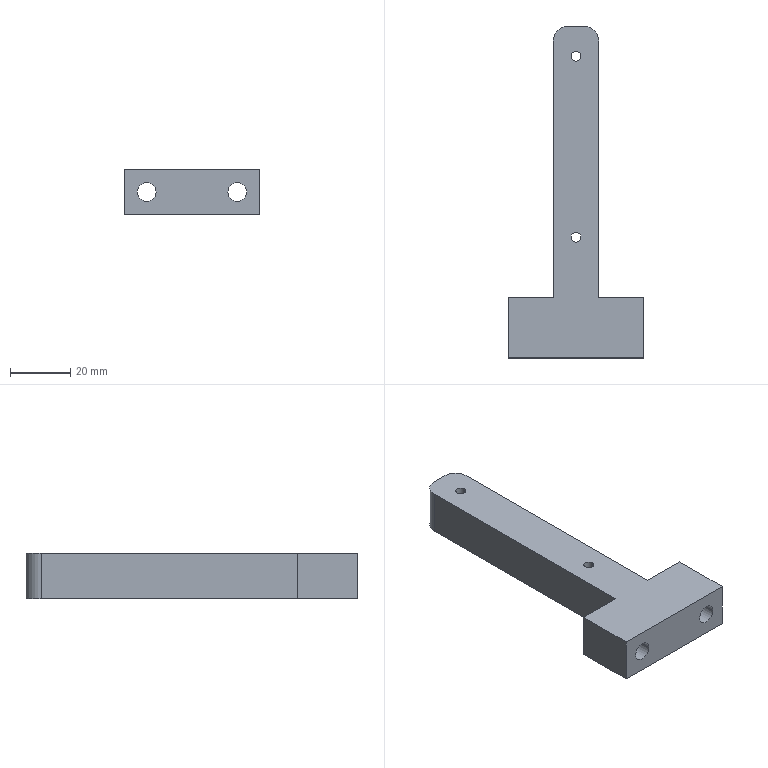Part | 1 solid | 26 faces | box 45 x 110 x 15 mm | volume 31351 mm3 | cylinder 14 | plane 12 | commonest cylinder face diameters 10 x6 3.3 x4 6.2 x4
STEP:
#1=CARTESIAN_POINT('',(20.85,100.,0.));
#2=VERTEX_POINT('',#1);
#3=CARTESIAN_POINT('',(24.15,100.,0.));
#4=VERTEX_POINT('',#3);
#5=CARTESIAN_POINT('',(22.5,100.,0.));
#6=DIRECTION('',(0.,0.,1.));
#7=DIRECTION('',(1.,0.,0.));
#8=AXIS2_PLACEMENT_3D('',#5,#6,#7);
#9=CIRCLE('',#8,1.65);
#10=EDGE_CURVE('',#2,#4,#9,.T.);
#11=ORIENTED_EDGE('',*,*,#10,.F.);
#12=CARTESIAN_POINT('',(20.85,100.,15.));
#13=VERTEX_POINT('',#12);
#14=CARTESIAN_POINT('',(20.85,100.,15.));
#15=DIRECTION('',(0.,0.,1.));
#16=VECTOR('',#15,1000.);
#17=LINE('',#14,#16);
#18=EDGE_CURVE('',#2,#13,#17,.T.);
#19=ORIENTED_EDGE('',*,*,#18,.T.);
#20=CARTESIAN_POINT('',(24.15,100.,15.));
#21=VERTEX_POINT('',#20);
#22=CARTESIAN_POINT('',(22.5,100.,15.));
#23=DIRECTION('',(0.,0.,1.));
#24=DIRECTION('',(1.,0.,0.));
#25=AXIS2_PLACEMENT_3D('',#22,#23,#24);
#26=CIRCLE('',#25,1.65);
#27=EDGE_CURVE('',#13,#21,#26,.T.);
#28=ORIENTED_EDGE('',*,*,#27,.T.);
#29=CARTESIAN_POINT('',(24.15,100.,15.));
#30=DIRECTION('',(0.,0.,1.));
#31=VECTOR('',#30,1000.);
#32=LINE('',#29,#31);
#33=EDGE_CURVE('',#4,#21,#32,.T.);
#34=ORIENTED_EDGE('',*,*,#33,.F.);
#35=EDGE_LOOP('',(#11,#19,#28,#34));
#36=FACE_OUTER_BOUND('',#35,.T.);
#37=CARTESIAN_POINT('',(22.5,100.,15.));
#38=DIRECTION('',(0.,0.,1.));
#39=DIRECTION('',(1.,0.,0.));
#40=AXIS2_PLACEMENT_3D('',#37,#38,#39);
#41=CYLINDRICAL_SURFACE('',#40,1.65);
#42=ADVANCED_FACE('',(#36),#41,.F.);
#43=CARTESIAN_POINT('',(20.85,40.,0.));
#44=VERTEX_POINT('',#43);
#45=CARTESIAN_POINT('',(24.15,40.,0.));
#46=VERTEX_POINT('',#45);
#47=CARTESIAN_POINT('',(22.5,40.,0.));
#48=DIRECTION('',(0.,0.,1.));
#49=DIRECTION('',(1.,0.,0.));
#50=AXIS2_PLACEMENT_3D('',#47,#48,#49);
#51=CIRCLE('',#50,1.65);
#52=EDGE_CURVE('',#44,#46,#51,.T.);
#53=ORIENTED_EDGE('',*,*,#52,.F.);
#54=CARTESIAN_POINT('',(20.85,40.,15.));
#55=VERTEX_POINT('',#54);
#56=CARTESIAN_POINT('',(20.85,40.,15.));
#57=DIRECTION('',(0.,0.,1.));
#58=VECTOR('',#57,1000.);
#59=LINE('',#56,#58);
#60=EDGE_CURVE('',#44,#55,#59,.T.);
#61=ORIENTED_EDGE('',*,*,#60,.T.);
#62=CARTESIAN_POINT('',(24.15,40.,15.));
#63=VERTEX_POINT('',#62);
#64=CARTESIAN_POINT('',(22.5,40.,15.));
#65=DIRECTION('',(0.,0.,1.));
#66=DIRECTION('',(1.,0.,0.));
#67=AXIS2_PLACEMENT_3D('',#64,#65,#66);
#68=CIRCLE('',#67,1.65);
#69=EDGE_CURVE('',#55,#63,#68,.T.);
#70=ORIENTED_EDGE('',*,*,#69,.T.);
#71=CARTESIAN_POINT('',(24.15,40.,15.));
#72=DIRECTION('',(0.,0.,1.));
#73=VECTOR('',#72,1000.);
#74=LINE('',#71,#73);
#75=EDGE_CURVE('',#46,#63,#74,.T.);
#76=ORIENTED_EDGE('',*,*,#75,.F.);
#77=EDGE_LOOP('',(#53,#61,#70,#76));
#78=FACE_OUTER_BOUND('',#77,.T.);
#79=CARTESIAN_POINT('',(22.5,40.,15.));
#80=DIRECTION('',(0.,0.,1.));
#81=DIRECTION('',(1.,0.,0.));
#82=AXIS2_PLACEMENT_3D('',#79,#80,#81);
#83=CYLINDRICAL_SURFACE('',#82,1.65);
#84=ADVANCED_FACE('',(#78),#83,.F.);
#85=CARTESIAN_POINT('',(12.5,12.,7.5));
#86=VERTEX_POINT('',#85);
#87=CARTESIAN_POINT('',(2.5,12.,7.5));
#88=VERTEX_POINT('',#87);
#89=CARTESIAN_POINT('',(7.5,12.,7.5));
#90=DIRECTION('',(0.,1.,0.));
#91=DIRECTION('',(-1.,0.,0.));
#92=AXIS2_PLACEMENT_3D('',#89,#90,#91);
#93=CIRCLE('',#92,5.);
#94=EDGE_CURVE('',#86,#88,#93,.T.);
#95=ORIENTED_EDGE('',*,*,#94,.F.);
#96=CARTESIAN_POINT('',(12.5,20.,7.5));
#97=VERTEX_POINT('',#96);
#98=CARTESIAN_POINT('',(12.5,12.,7.5));
#99=DIRECTION('',(0.,1.,0.));
#100=VECTOR('',#99,1000.);
#101=LINE('',#98,#100);
#102=EDGE_CURVE('',#86,#97,#101,.T.);
#103=ORIENTED_EDGE('',*,*,#102,.T.);
#104=CARTESIAN_POINT('',(2.5,20.,7.5));
#105=VERTEX_POINT('',#104);
#106=CARTESIAN_POINT('',(7.5,20.,7.5));
#107=DIRECTION('',(0.,1.,0.));
#108=DIRECTION('',(-1.,0.,0.));
#109=AXIS2_PLACEMENT_3D('',#106,#107,#108);
#110=CIRCLE('',#109,5.);
#111=EDGE_CURVE('',#97,#105,#110,.T.);
#112=ORIENTED_EDGE('',*,*,#111,.T.);
#113=CARTESIAN_POINT('',(2.5,12.,7.5));
#114=DIRECTION('',(0.,1.,0.));
#115=VECTOR('',#114,1000.);
#116=LINE('',#113,#115);
#117=EDGE_CURVE('',#88,#105,#116,.T.);
#118=ORIENTED_EDGE('',*,*,#117,.F.);
#119=EDGE_LOOP('',(#95,#103,#112,#118));
#120=FACE_OUTER_BOUND('',#119,.T.);
#121=CARTESIAN_POINT('',(7.5,12.,7.5));
#122=DIRECTION('',(0.,1.,0.));
#123=DIRECTION('',(-1.,0.,0.));
#124=AXIS2_PLACEMENT_3D('',#121,#122,#123);
#125=CYLINDRICAL_SURFACE('',#124,5.);
#126=ADVANCED_FACE('',(#120),#125,.F.);
#127=CARTESIAN_POINT('',(42.5,12.,7.5));
#128=VERTEX_POINT('',#127);
#129=CARTESIAN_POINT('',(32.5,12.,7.5));
#130=VERTEX_POINT('',#129);
#131=CARTESIAN_POINT('',(37.5,12.,7.5));
#132=DIRECTION('',(0.,1.,0.));
#133=DIRECTION('',(1.,0.,0.));
#134=AXIS2_PLACEMENT_3D('',#131,#132,#133);
#135=CIRCLE('',#134,5.);
#136=EDGE_CURVE('',#128,#130,#135,.T.);
#137=ORIENTED_EDGE('',*,*,#136,.F.);
#138=CARTESIAN_POINT('',(42.5,20.,7.5));
#139=VERTEX_POINT('',#138);
#140=CARTESIAN_POINT('',(42.5,12.,7.5));
#141=DIRECTION('',(0.,1.,0.));
#142=VECTOR('',#141,1000.);
#143=LINE('',#140,#142);
#144=EDGE_CURVE('',#128,#139,#143,.T.);
#145=ORIENTED_EDGE('',*,*,#144,.T.);
#146=CARTESIAN_POINT('',(32.5,20.,7.5));
#147=VERTEX_POINT('',#146);
#148=CARTESIAN_POINT('',(37.5,20.,7.5));
#149=DIRECTION('',(0.,1.,0.));
#150=DIRECTION('',(1.,0.,0.));
#151=AXIS2_PLACEMENT_3D('',#148,#149,#150);
#152=CIRCLE('',#151,5.);
#153=EDGE_CURVE('',#139,#147,#152,.T.);
#154=ORIENTED_EDGE('',*,*,#153,.T.);
#155=CARTESIAN_POINT('',(32.5,12.,7.5));
#156=DIRECTION('',(0.,1.,0.));
#157=VECTOR('',#156,1000.);
#158=LINE('',#155,#157);
#159=EDGE_CURVE('',#130,#147,#158,.T.);
#160=ORIENTED_EDGE('',*,*,#159,.F.);
#161=EDGE_LOOP('',(#137,#145,#154,#160));
#162=FACE_OUTER_BOUND('',#161,.T.);
#163=CARTESIAN_POINT('',(37.5,12.,7.5));
#164=DIRECTION('',(0.,1.,0.));
#165=DIRECTION('',(-1.,0.,0.));
#166=AXIS2_PLACEMENT_3D('',#163,#164,#165);
#167=CYLINDRICAL_SURFACE('',#166,5.);
#168=ADVANCED_FACE('',(#162),#167,.F.);
#169=CARTESIAN_POINT('',(40.6,0.,7.5));
#170=VERTEX_POINT('',#169);
#171=CARTESIAN_POINT('',(34.4,0.,7.5));
#172=VERTEX_POINT('',#171);
#173=CARTESIAN_POINT('',(37.5,0.,7.5));
#174=DIRECTION('',(0.,1.,0.));
#175=DIRECTION('',(1.,0.,0.));
#176=AXIS2_PLACEMENT_3D('',#173,#174,#175);
#177=CIRCLE('',#176,3.1);
#178=EDGE_CURVE('',#170,#172,#177,.T.);
#179=ORIENTED_EDGE('',*,*,#178,.F.);
#180=CARTESIAN_POINT('',(40.6,12.,7.5));
#181=VERTEX_POINT('',#180);
#182=CARTESIAN_POINT('',(40.6,0.,7.5));
#183=DIRECTION('',(0.,1.,0.));
#184=VECTOR('',#183,1000.);
#185=LINE('',#182,#184);
#186=EDGE_CURVE('',#170,#181,#185,.T.);
#187=ORIENTED_EDGE('',*,*,#186,.T.);
#188=CARTESIAN_POINT('',(34.4,12.,7.5));
#189=VERTEX_POINT('',#188);
#190=CARTESIAN_POINT('',(37.5,12.,7.5));
#191=DIRECTION('',(0.,1.,0.));
#192=DIRECTION('',(1.,0.,0.));
#193=AXIS2_PLACEMENT_3D('',#190,#191,#192);
#194=CIRCLE('',#193,3.1);
#195=EDGE_CURVE('',#181,#189,#194,.T.);
#196=ORIENTED_EDGE('',*,*,#195,.T.);
#197=CARTESIAN_POINT('',(34.4,0.,7.5));
#198=DIRECTION('',(0.,1.,0.));
#199=VECTOR('',#198,1000.);
#200=LINE('',#197,#199);
#201=EDGE_CURVE('',#172,#189,#200,.T.);
#202=ORIENTED_EDGE('',*,*,#201,.F.);
#203=EDGE_LOOP('',(#179,#187,#196,#202));
#204=FACE_OUTER_BOUND('',#203,.T.);
#205=CARTESIAN_POINT('',(37.5,0.,7.5));
#206=DIRECTION('',(0.,1.,0.));
#207=DIRECTION('',(-1.,0.,0.));
#208=AXIS2_PLACEMENT_3D('',#205,#206,#207);
#209=CYLINDRICAL_SURFACE('',#208,3.1);
#210=ADVANCED_FACE('',(#204),#209,.F.);
#211=CARTESIAN_POINT('',(10.6,0.,7.5));
#212=VERTEX_POINT('',#211);
#213=CARTESIAN_POINT('',(4.4,0.,7.5));
#214=VERTEX_POINT('',#213);
#215=CARTESIAN_POINT('',(7.5,0.,7.5));
#216=DIRECTION('',(0.,1.,0.));
#217=DIRECTION('',(-1.,0.,0.));
#218=AXIS2_PLACEMENT_3D('',#215,#216,#217);
#219=CIRCLE('',#218,3.1);
#220=EDGE_CURVE('',#212,#214,#219,.T.);
#221=ORIENTED_EDGE('',*,*,#220,.F.);
#222=CARTESIAN_POINT('',(10.6,12.,7.5));
#223=VERTEX_POINT('',#222);
#224=CARTESIAN_POINT('',(10.6,0.,7.5));
#225=DIRECTION('',(0.,1.,0.));
#226=VECTOR('',#225,1000.);
#227=LINE('',#224,#226);
#228=EDGE_CURVE('',#212,#223,#227,.T.);
#229=ORIENTED_EDGE('',*,*,#228,.T.);
#230=CARTESIAN_POINT('',(4.4,12.,7.5));
#231=VERTEX_POINT('',#230);
#232=CARTESIAN_POINT('',(7.5,12.,7.5));
#233=DIRECTION('',(0.,-1.,0.));
#234=DIRECTION('',(-1.,0.,0.));
#235=AXIS2_PLACEMENT_3D('',#232,#233,#234);
#236=CIRCLE('',#235,3.1);
#237=EDGE_CURVE('',#231,#223,#236,.T.);
#238=ORIENTED_EDGE('',*,*,#237,.F.);
#239=CARTESIAN_POINT('',(4.4,0.,7.5));
#240=DIRECTION('',(0.,1.,0.));
#241=VECTOR('',#240,1000.);
#242=LINE('',#239,#241);
#243=EDGE_CURVE('',#214,#231,#242,.T.);
#244=ORIENTED_EDGE('',*,*,#243,.F.);
#245=EDGE_LOOP('',(#221,#229,#238,#244));
#246=FACE_OUTER_BOUND('',#245,.T.);
#247=CARTESIAN_POINT('',(7.5,0.,7.5));
#248=DIRECTION('',(0.,1.,0.));
#249=DIRECTION('',(-1.,0.,0.));
#250=AXIS2_PLACEMENT_3D('',#247,#248,#249);
#251=CYLINDRICAL_SURFACE('',#250,3.1);
#252=ADVANCED_FACE('',(#246),#251,.F.);
#253=ORIENTED_EDGE('',*,*,#228,.F.);
#254=CARTESIAN_POINT('',(7.5,0.,7.5));
#255=DIRECTION('',(0.,1.,0.));
#256=DIRECTION('',(-1.,0.,0.));
#257=AXIS2_PLACEMENT_3D('',#254,#255,#256);
#258=CIRCLE('',#257,3.1);
#259=EDGE_CURVE('',#214,#212,#258,.T.);
#260=ORIENTED_EDGE('',*,*,#259,.F.);
#261=ORIENTED_EDGE('',*,*,#243,.T.);
#262=CARTESIAN_POINT('',(7.5,12.,7.5));
#263=DIRECTION('',(0.,-1.,0.));
#264=DIRECTION('',(-1.,0.,0.));
#265=AXIS2_PLACEMENT_3D('',#262,#263,#264);
#266=CIRCLE('',#265,3.1);
#267=EDGE_CURVE('',#223,#231,#266,.T.);
#268=ORIENTED_EDGE('',*,*,#267,.F.);
#269=EDGE_LOOP('',(#253,#260,#261,#268));
#270=FACE_OUTER_BOUND('',#269,.T.);
#271=CARTESIAN_POINT('',(7.5,0.,7.5));
#272=DIRECTION('',(0.,1.,0.));
#273=DIRECTION('',(-1.,0.,0.));
#274=AXIS2_PLACEMENT_3D('',#271,#272,#273);
#275=CYLINDRICAL_SURFACE('',#274,3.1);
#276=ADVANCED_FACE('',(#270),#275,.F.);
#277=CARTESIAN_POINT('',(0.,20.,15.));
#278=VERTEX_POINT('',#277);
#279=CARTESIAN_POINT('',(0.,0.,15.));
#280=VERTEX_POINT('',#279);
#281=CARTESIAN_POINT('',(0.,0.,15.));
#282=DIRECTION('',(0.,-1.,0.));
#283=VECTOR('',#282,1000.);
#284=LINE('',#281,#283);
#285=EDGE_CURVE('',#278,#280,#284,.T.);
#286=ORIENTED_EDGE('',*,*,#285,.F.);
#287=CARTESIAN_POINT('',(0.,20.,0.));
#288=VERTEX_POINT('',#287);
#289=CARTESIAN_POINT('',(0.,20.,0.));
#290=DIRECTION('',(0.,0.,1.));
#291=VECTOR('',#290,1000.);
#292=LINE('',#289,#291);
#293=EDGE_CURVE('',#288,#278,#292,.T.);
#294=ORIENTED_EDGE('',*,*,#293,.F.);
#295=CARTESIAN_POINT('',(0.,0.,0.));
#296=VERTEX_POINT('',#295);
#297=CARTESIAN_POINT('',(0.,0.,0.));
#298=DIRECTION('',(0.,-1.,0.));
#299=VECTOR('',#298,1000.);
#300=LINE('',#297,#299);
#301=EDGE_CURVE('',#288,#296,#300,.T.);
#302=ORIENTED_EDGE('',*,*,#301,.T.);
#303=CARTESIAN_POINT('',(0.,0.,15.));
#304=DIRECTION('',(0.,0.,-1.));
#305=VECTOR('',#304,1000.);
#306=LINE('',#303,#305);
#307=EDGE_CURVE('',#280,#296,#306,.T.);
#308=ORIENTED_EDGE('',*,*,#307,.F.);
#309=EDGE_LOOP('',(#286,#294,#302,#308));
#310=FACE_OUTER_BOUND('',#309,.T.);
#311=CARTESIAN_POINT('',(0.,0.,15.));
#312=DIRECTION('',(1.,0.,0.));
#313=DIRECTION('',(0.,0.,-1.));
#314=AXIS2_PLACEMENT_3D('',#311,#312,#313);
#315=PLANE('',#314);
#316=ADVANCED_FACE('',(#310),#315,.F.);
#317=ORIENTED_EDGE('',*,*,#259,.T.);
#318=ORIENTED_EDGE('',*,*,#220,.T.);
#319=EDGE_LOOP('',(#317,#318));
#320=FACE_BOUND('',#319,.T.);
#321=CARTESIAN_POINT('',(37.5,0.,7.5));
#322=DIRECTION('',(0.,1.,0.));
#323=DIRECTION('',(1.,0.,0.));
#324=AXIS2_PLACEMENT_3D('',#321,#322,#323);
#325=CIRCLE('',#324,3.1);
#326=EDGE_CURVE('',#172,#170,#325,.T.);
#327=ORIENTED_EDGE('',*,*,#326,.T.);
#328=ORIENTED_EDGE('',*,*,#178,.T.);
#329=EDGE_LOOP('',(#327,#328));
#330=FACE_BOUND('',#329,.T.);
#331=CARTESIAN_POINT('',(45.,0.,0.));
#332=VERTEX_POINT('',#331);
#333=CARTESIAN_POINT('',(0.,0.,0.));
#334=DIRECTION('',(1.,0.,0.));
#335=VECTOR('',#334,1000.);
#336=LINE('',#333,#335);
#337=EDGE_CURVE('',#296,#332,#336,.T.);
#338=ORIENTED_EDGE('',*,*,#337,.T.);
#339=CARTESIAN_POINT('',(45.,0.,15.));
#340=VERTEX_POINT('',#339);
#341=CARTESIAN_POINT('',(45.,0.,15.));
#342=DIRECTION('',(0.,0.,-1.));
#343=VECTOR('',#342,1000.);
#344=LINE('',#341,#343);
#345=EDGE_CURVE('',#340,#332,#344,.T.);
#346=ORIENTED_EDGE('',*,*,#345,.F.);
#347=CARTESIAN_POINT('',(0.,0.,15.));
#348=DIRECTION('',(1.,0.,0.));
#349=VECTOR('',#348,1000.);
#350=LINE('',#347,#349);
#351=EDGE_CURVE('',#280,#340,#350,.T.);
#352=ORIENTED_EDGE('',*,*,#351,.F.);
#353=ORIENTED_EDGE('',*,*,#307,.T.);
#354=EDGE_LOOP('',(#338,#346,#352,#353));
#355=FACE_OUTER_BOUND('',#354,.T.);
#356=CARTESIAN_POINT('',(0.,0.,15.));
#357=DIRECTION('',(0.,1.,0.));
#358=DIRECTION('',(0.,0.,1.));
#359=AXIS2_PLACEMENT_3D('',#356,#357,#358);
#360=PLANE('',#359);
#361=ADVANCED_FACE('',(#320,#330,#355),#360,.F.);
#362=CARTESIAN_POINT('',(45.,20.,0.));
#363=VERTEX_POINT('',#362);
#364=CARTESIAN_POINT('',(45.,0.,0.));
#365=DIRECTION('',(0.,1.,0.));
#366=VECTOR('',#365,1000.);
#367=LINE('',#364,#366);
#368=EDGE_CURVE('',#332,#363,#367,.T.);
#369=ORIENTED_EDGE('',*,*,#368,.T.);
#370=CARTESIAN_POINT('',(45.,20.,15.));
#371=VERTEX_POINT('',#370);
#372=CARTESIAN_POINT('',(45.,20.,0.));
#373=DIRECTION('',(0.,0.,1.));
#374=VECTOR('',#373,1000.);
#375=LINE('',#372,#374);
#376=EDGE_CURVE('',#363,#371,#375,.T.);
#377=ORIENTED_EDGE('',*,*,#376,.T.);
#378=CARTESIAN_POINT('',(45.,0.,15.));
#379=DIRECTION('',(0.,1.,0.));
#380=VECTOR('',#379,1000.);
#381=LINE('',#378,#380);
#382=EDGE_CURVE('',#340,#371,#381,.T.);
#383=ORIENTED_EDGE('',*,*,#382,.F.);
#384=ORIENTED_EDGE('',*,*,#345,.T.);
#385=EDGE_LOOP('',(#369,#377,#383,#384));
#386=FACE_OUTER_BOUND('',#385,.T.);
#387=CARTESIAN_POINT('',(45.,0.,15.));
#388=DIRECTION('',(-1.,0.,0.));
#389=DIRECTION('',(0.,0.,1.));
#390=AXIS2_PLACEMENT_3D('',#387,#388,#389);
#391=PLANE('',#390);
#392=ADVANCED_FACE('',(#386),#391,.F.);
#393=CARTESIAN_POINT('',(25.,110.,15.));
#394=VERTEX_POINT('',#393);
#395=CARTESIAN_POINT('',(20.,110.,15.));
#396=VERTEX_POINT('',#395);
#397=CARTESIAN_POINT('',(0.,110.,15.));
#398=DIRECTION('',(-1.,0.,0.));
#399=VECTOR('',#398,1000.);
#400=LINE('',#397,#399);
#401=EDGE_CURVE('',#394,#396,#400,.T.);
#402=ORIENTED_EDGE('',*,*,#401,.F.);
#403=CARTESIAN_POINT('',(25.,110.,0.));
#404=VERTEX_POINT('',#403);
#405=CARTESIAN_POINT('',(25.,110.,15.));
#406=DIRECTION('',(0.,0.,-1.));
#407=VECTOR('',#406,1000.);
#408=LINE('',#405,#407);
#409=EDGE_CURVE('',#394,#404,#408,.T.);
#410=ORIENTED_EDGE('',*,*,#409,.T.);
#411=CARTESIAN_POINT('',(20.,110.,0.));
#412=VERTEX_POINT('',#411);
#413=CARTESIAN_POINT('',(0.,110.,0.));
#414=DIRECTION('',(-1.,0.,0.));
#415=VECTOR('',#414,1000.);
#416=LINE('',#413,#415);
#417=EDGE_CURVE('',#404,#412,#416,.T.);
#418=ORIENTED_EDGE('',*,*,#417,.T.);
#419=CARTESIAN_POINT('',(20.,110.,15.));
#420=DIRECTION('',(0.,0.,1.));
#421=VECTOR('',#420,1000.);
#422=LINE('',#419,#421);
#423=EDGE_CURVE('',#412,#396,#422,.T.);
#424=ORIENTED_EDGE('',*,*,#423,.T.);
#425=EDGE_LOOP('',(#402,#410,#418,#424));
#426=FACE_OUTER_BOUND('',#425,.T.);
#427=CARTESIAN_POINT('',(0.,110.,15.));
#428=DIRECTION('',(0.,-1.,0.));
#429=DIRECTION('',(0.,0.,-1.));
#430=AXIS2_PLACEMENT_3D('',#427,#428,#429);
#431=PLANE('',#430);
#432=ADVANCED_FACE('',(#426),#431,.F.);
#433=CARTESIAN_POINT('',(22.5,100.,15.));
#434=DIRECTION('',(0.,0.,1.));
#435=DIRECTION('',(1.,0.,0.));
#436=AXIS2_PLACEMENT_3D('',#433,#434,#435);
#437=CIRCLE('',#436,1.65);
#438=EDGE_CURVE('',#21,#13,#437,.T.);
#439=ORIENTED_EDGE('',*,*,#438,.F.);
#440=ORIENTED_EDGE('',*,*,#27,.F.);
#441=EDGE_LOOP('',(#439,#440));
#442=FACE_BOUND('',#441,.T.);
#443=CARTESIAN_POINT('',(22.5,40.,15.));
#444=DIRECTION('',(0.,0.,1.));
#445=DIRECTION('',(1.,0.,0.));
#446=AXIS2_PLACEMENT_3D('',#443,#444,#445);
#447=CIRCLE('',#446,1.65);
#448=EDGE_CURVE('',#63,#55,#447,.T.);
#449=ORIENTED_EDGE('',*,*,#448,.F.);
#450=ORIENTED_EDGE('',*,*,#69,.F.);
#451=EDGE_LOOP('',(#449,#450));
#452=FACE_BOUND('',#451,.T.);
#453=CARTESIAN_POINT('',(30.,105.,15.));
#454=VERTEX_POINT('',#453);
#455=CARTESIAN_POINT('',(30.,20.,15.));
#456=VERTEX_POINT('',#455);
#457=CARTESIAN_POINT('',(30.,110.,15.));
#458=DIRECTION('',(0.,-1.,0.));
#459=VECTOR('',#458,1000.);
#460=LINE('',#457,#459);
#461=EDGE_CURVE('',#454,#456,#460,.T.);
#462=ORIENTED_EDGE('',*,*,#461,.F.);
#463=CARTESIAN_POINT('',(25.,105.,15.));
#464=DIRECTION('',(0.,0.,1.));
#465=DIRECTION('',(-1.,0.,0.));
#466=AXIS2_PLACEMENT_3D('',#463,#464,#465);
#467=CIRCLE('',#466,5.);
#468=EDGE_CURVE('',#454,#394,#467,.T.);
#469=ORIENTED_EDGE('',*,*,#468,.T.);
#470=ORIENTED_EDGE('',*,*,#401,.T.);
#471=CARTESIAN_POINT('',(15.,105.,15.));
#472=VERTEX_POINT('',#471);
#473=CARTESIAN_POINT('',(20.,105.,15.));
#474=DIRECTION('',(0.,0.,1.));
#475=DIRECTION('',(-1.,0.,0.));
#476=AXIS2_PLACEMENT_3D('',#473,#474,#475);
#477=CIRCLE('',#476,5.);
#478=EDGE_CURVE('',#396,#472,#477,.T.);
#479=ORIENTED_EDGE('',*,*,#478,.T.);
#480=CARTESIAN_POINT('',(15.,20.,15.));
#481=VERTEX_POINT('',#480);
#482=CARTESIAN_POINT('',(15.,110.,15.));
#483=DIRECTION('',(0.,1.,0.));
#484=VECTOR('',#483,1000.);
#485=LINE('',#482,#484);
#486=EDGE_CURVE('',#481,#472,#485,.T.);
#487=ORIENTED_EDGE('',*,*,#486,.F.);
#488=CARTESIAN_POINT('',(0.,20.,15.));
#489=DIRECTION('',(1.,0.,0.));
#490=VECTOR('',#489,1000.);
#491=LINE('',#488,#490);
#492=EDGE_CURVE('',#278,#481,#491,.T.);
#493=ORIENTED_EDGE('',*,*,#492,.F.);
#494=ORIENTED_EDGE('',*,*,#285,.T.);
#495=ORIENTED_EDGE('',*,*,#351,.T.);
#496=ORIENTED_EDGE('',*,*,#382,.T.);
#497=CARTESIAN_POINT('',(45.,20.,15.));
#498=DIRECTION('',(1.,0.,0.));
#499=VECTOR('',#498,1000.);
#500=LINE('',#497,#499);
#501=EDGE_CURVE('',#456,#371,#500,.T.);
#502=ORIENTED_EDGE('',*,*,#501,.F.);
#503=EDGE_LOOP('',(#462,#469,#470,#479,#487,#493,#494,#495,#496,#502));
#504=FACE_OUTER_BOUND('',#503,.T.);
#505=CARTESIAN_POINT('',(0.,0.,15.));
#506=DIRECTION('',(0.,0.,-1.));
#507=DIRECTION('',(-1.,0.,0.));
#508=AXIS2_PLACEMENT_3D('',#505,#506,#507);
#509=PLANE('',#508);
#510=ADVANCED_FACE('',(#442,#452,#504),#509,.F.);
#511=CARTESIAN_POINT('',(22.5,100.,0.));
#512=DIRECTION('',(0.,0.,1.));
#513=DIRECTION('',(1.,0.,0.));
#514=AXIS2_PLACEMENT_3D('',#511,#512,#513);
#515=CIRCLE('',#514,1.65);
#516=EDGE_CURVE('',#4,#2,#515,.T.);
#517=ORIENTED_EDGE('',*,*,#516,.T.);
#518=ORIENTED_EDGE('',*,*,#10,.T.);
#519=EDGE_LOOP('',(#517,#518));
#520=FACE_BOUND('',#519,.T.);
#521=CARTESIAN_POINT('',(22.5,40.,0.));
#522=DIRECTION('',(0.,0.,1.));
#523=DIRECTION('',(1.,0.,0.));
#524=AXIS2_PLACEMENT_3D('',#521,#522,#523);
#525=CIRCLE('',#524,1.65);
#526=EDGE_CURVE('',#46,#44,#525,.T.);
#527=ORIENTED_EDGE('',*,*,#526,.T.);
#528=ORIENTED_EDGE('',*,*,#52,.T.);
#529=EDGE_LOOP('',(#527,#528));
#530=FACE_BOUND('',#529,.T.);
#531=ORIENTED_EDGE('',*,*,#417,.F.);
#532=CARTESIAN_POINT('',(30.,105.,0.));
#533=VERTEX_POINT('',#532);
#534=CARTESIAN_POINT('',(25.,105.,0.));
#535=DIRECTION('',(0.,0.,-1.));
#536=DIRECTION('',(-1.,0.,0.));
#537=AXIS2_PLACEMENT_3D('',#534,#535,#536);
#538=CIRCLE('',#537,5.);
#539=EDGE_CURVE('',#404,#533,#538,.T.);
#540=ORIENTED_EDGE('',*,*,#539,.T.);
#541=CARTESIAN_POINT('',(30.,20.,0.));
#542=VERTEX_POINT('',#541);
#543=CARTESIAN_POINT('',(30.,110.,0.));
#544=DIRECTION('',(0.,-1.,0.));
#545=VECTOR('',#544,1000.);
#546=LINE('',#543,#545);
#547=EDGE_CURVE('',#533,#542,#546,.T.);
#548=ORIENTED_EDGE('',*,*,#547,.T.);
#549=CARTESIAN_POINT('',(45.,20.,0.));
#550=DIRECTION('',(1.,0.,0.));
#551=VECTOR('',#550,1000.);
#552=LINE('',#549,#551);
#553=EDGE_CURVE('',#542,#363,#552,.T.);
#554=ORIENTED_EDGE('',*,*,#553,.T.);
#555=ORIENTED_EDGE('',*,*,#368,.F.);
#556=ORIENTED_EDGE('',*,*,#337,.F.);
#557=ORIENTED_EDGE('',*,*,#301,.F.);
#558=CARTESIAN_POINT('',(15.,20.,0.));
#559=VERTEX_POINT('',#558);
#560=CARTESIAN_POINT('',(0.,20.,0.));
#561=DIRECTION('',(1.,0.,0.));
#562=VECTOR('',#561,1000.);
#563=LINE('',#560,#562);
#564=EDGE_CURVE('',#288,#559,#563,.T.);
#565=ORIENTED_EDGE('',*,*,#564,.T.);
#566=CARTESIAN_POINT('',(15.,105.,0.));
#567=VERTEX_POINT('',#566);
#568=CARTESIAN_POINT('',(15.,110.,0.));
#569=DIRECTION('',(0.,1.,0.));
#570=VECTOR('',#569,1000.);
#571=LINE('',#568,#570);
#572=EDGE_CURVE('',#559,#567,#571,.T.);
#573=ORIENTED_EDGE('',*,*,#572,.T.);
#574=CARTESIAN_POINT('',(20.,105.,0.));
#575=DIRECTION('',(0.,0.,-1.));
#576=DIRECTION('',(-1.,0.,0.));
#577=AXIS2_PLACEMENT_3D('',#574,#575,#576);
#578=CIRCLE('',#577,5.);
#579=EDGE_CURVE('',#567,#412,#578,.T.);
#580=ORIENTED_EDGE('',*,*,#579,.T.);
#581=EDGE_LOOP('',(#531,#540,#548,#554,#555,#556,#557,#565,#573,#580));
#582=FACE_OUTER_BOUND('',#581,.T.);
#583=CARTESIAN_POINT('',(0.,0.,0.));
#584=DIRECTION('',(0.,0.,-1.));
#585=DIRECTION('',(-1.,0.,0.));
#586=AXIS2_PLACEMENT_3D('',#583,#584,#585);
#587=PLANE('',#586);
#588=ADVANCED_FACE('',(#520,#530,#582),#587,.T.);
#589=CARTESIAN_POINT('',(37.5,20.,7.5));
#590=DIRECTION('',(0.,1.,0.));
#591=DIRECTION('',(1.,0.,0.));
#592=AXIS2_PLACEMENT_3D('',#589,#590,#591);
#593=CIRCLE('',#592,5.);
#594=EDGE_CURVE('',#147,#139,#593,.T.);
#595=ORIENTED_EDGE('',*,*,#594,.F.);
#596=ORIENTED_EDGE('',*,*,#153,.F.);
#597=EDGE_LOOP('',(#595,#596));
#598=FACE_BOUND('',#597,.T.);
#599=ORIENTED_EDGE('',*,*,#501,.T.);
#600=ORIENTED_EDGE('',*,*,#376,.F.);
#601=ORIENTED_EDGE('',*,*,#553,.F.);
#602=CARTESIAN_POINT('',(30.,20.,0.));
#603=DIRECTION('',(0.,0.,1.));
#604=VECTOR('',#603,1000.);
#605=LINE('',#602,#604);
#606=EDGE_CURVE('',#542,#456,#605,.T.);
#607=ORIENTED_EDGE('',*,*,#606,.T.);
#608=EDGE_LOOP('',(#599,#600,#601,#607));
#609=FACE_OUTER_BOUND('',#608,.T.);
#610=CARTESIAN_POINT('',(45.,20.,0.));
#611=DIRECTION('',(0.,-1.,0.));
#612=DIRECTION('',(1.,0.,0.));
#613=AXIS2_PLACEMENT_3D('',#610,#611,#612);
#614=PLANE('',#613);
#615=ADVANCED_FACE('',(#598,#609),#614,.F.);
#616=ORIENTED_EDGE('',*,*,#547,.F.);
#617=CARTESIAN_POINT('',(30.,105.,0.));
#618=DIRECTION('',(0.,0.,1.));
#619=VECTOR('',#618,1000.);
#620=LINE('',#617,#619);
#621=EDGE_CURVE('',#533,#454,#620,.T.);
#622=ORIENTED_EDGE('',*,*,#621,.T.);
#623=ORIENTED_EDGE('',*,*,#461,.T.);
#624=ORIENTED_EDGE('',*,*,#606,.F.);
#625=EDGE_LOOP('',(#616,#622,#623,#624));
#626=FACE_OUTER_BOUND('',#625,.T.);
#627=CARTESIAN_POINT('',(30.,110.,0.));
#628=DIRECTION('',(-1.,0.,0.));
#629=DIRECTION('',(0.,-1.,0.));
#630=AXIS2_PLACEMENT_3D('',#627,#628,#629);
#631=PLANE('',#630);
#632=ADVANCED_FACE('',(#626),#631,.F.);
#633=ORIENTED_EDGE('',*,*,#486,.T.);
#634=CARTESIAN_POINT('',(15.,105.,0.));
#635=DIRECTION('',(0.,0.,-1.));
#636=VECTOR('',#635,1000.);
#637=LINE('',#634,#636);
#638=EDGE_CURVE('',#472,#567,#637,.T.);
#639=ORIENTED_EDGE('',*,*,#638,.T.);
#640=ORIENTED_EDGE('',*,*,#572,.F.);
#641=CARTESIAN_POINT('',(15.,20.,0.));
#642=DIRECTION('',(0.,0.,1.));
#643=VECTOR('',#642,1000.);
#644=LINE('',#641,#643);
#645=EDGE_CURVE('',#559,#481,#644,.T.);
#646=ORIENTED_EDGE('',*,*,#645,.T.);
#647=EDGE_LOOP('',(#633,#639,#640,#646));
#648=FACE_OUTER_BOUND('',#647,.T.);
#649=CARTESIAN_POINT('',(15.,110.,0.));
#650=DIRECTION('',(1.,0.,0.));
#651=DIRECTION('',(0.,1.,0.));
#652=AXIS2_PLACEMENT_3D('',#649,#650,#651);
#653=PLANE('',#652);
#654=ADVANCED_FACE('',(#648),#653,.F.);
#655=CARTESIAN_POINT('',(7.5,20.,7.5));
#656=DIRECTION('',(0.,1.,0.));
#657=DIRECTION('',(-1.,0.,0.));
#658=AXIS2_PLACEMENT_3D('',#655,#656,#657);
#659=CIRCLE('',#658,5.);
#660=EDGE_CURVE('',#105,#97,#659,.T.);
#661=ORIENTED_EDGE('',*,*,#660,.F.);
#662=ORIENTED_EDGE('',*,*,#111,.F.);
#663=EDGE_LOOP('',(#661,#662));
#664=FACE_BOUND('',#663,.T.);
#665=ORIENTED_EDGE('',*,*,#492,.T.);
#666=ORIENTED_EDGE('',*,*,#645,.F.);
#667=ORIENTED_EDGE('',*,*,#564,.F.);
#668=ORIENTED_EDGE('',*,*,#293,.T.);
#669=EDGE_LOOP('',(#665,#666,#667,#668));
#670=FACE_OUTER_BOUND('',#669,.T.);
#671=CARTESIAN_POINT('',(0.,20.,0.));
#672=DIRECTION('',(0.,-1.,0.));
#673=DIRECTION('',(1.,0.,0.));
#674=AXIS2_PLACEMENT_3D('',#671,#672,#673);
#675=PLANE('',#674);
#676=ADVANCED_FACE('',(#664,#670),#675,.F.);
#677=ORIENTED_EDGE('',*,*,#186,.F.);
#678=ORIENTED_EDGE('',*,*,#326,.F.);
#679=ORIENTED_EDGE('',*,*,#201,.T.);
#680=CARTESIAN_POINT('',(37.5,12.,7.5));
#681=DIRECTION('',(0.,1.,0.));
#682=DIRECTION('',(1.,0.,0.));
#683=AXIS2_PLACEMENT_3D('',#680,#681,#682);
#684=CIRCLE('',#683,3.1);
#685=EDGE_CURVE('',#189,#181,#684,.T.);
#686=ORIENTED_EDGE('',*,*,#685,.T.);
#687=EDGE_LOOP('',(#677,#678,#679,#686));
#688=FACE_OUTER_BOUND('',#687,.T.);
#689=CARTESIAN_POINT('',(37.5,0.,7.5));
#690=DIRECTION('',(0.,1.,0.));
#691=DIRECTION('',(-1.,0.,0.));
#692=AXIS2_PLACEMENT_3D('',#689,#690,#691);
#693=CYLINDRICAL_SURFACE('',#692,3.1);
#694=ADVANCED_FACE('',(#688),#693,.F.);
#695=CARTESIAN_POINT('',(37.5,12.,7.5));
#696=DIRECTION('',(0.,1.,0.));
#697=DIRECTION('',(1.,0.,0.));
#698=AXIS2_PLACEMENT_3D('',#695,#696,#697);
#699=CIRCLE('',#698,5.);
#700=EDGE_CURVE('',#130,#128,#699,.T.);
#701=ORIENTED_EDGE('',*,*,#700,.T.);
#702=ORIENTED_EDGE('',*,*,#136,.T.);
#703=EDGE_LOOP('',(#701,#702));
#704=FACE_OUTER_BOUND('',#703,.T.);
#705=ORIENTED_EDGE('',*,*,#685,.F.);
#706=ORIENTED_EDGE('',*,*,#195,.F.);
#707=EDGE_LOOP('',(#705,#706));
#708=FACE_BOUND('',#707,.T.);
#709=CARTESIAN_POINT('',(37.5,12.,7.5));
#710=DIRECTION('',(0.,-1.,0.));
#711=DIRECTION('',(1.,0.,0.));
#712=AXIS2_PLACEMENT_3D('',#709,#710,#711);
#713=PLANE('',#712);
#714=ADVANCED_FACE('',(#704,#708),#713,.F.);
#715=ORIENTED_EDGE('',*,*,#144,.F.);
#716=ORIENTED_EDGE('',*,*,#700,.F.);
#717=ORIENTED_EDGE('',*,*,#159,.T.);
#718=ORIENTED_EDGE('',*,*,#594,.T.);
#719=EDGE_LOOP('',(#715,#716,#717,#718));
#720=FACE_OUTER_BOUND('',#719,.T.);
#721=CARTESIAN_POINT('',(37.5,12.,7.5));
#722=DIRECTION('',(0.,1.,0.));
#723=DIRECTION('',(-1.,0.,0.));
#724=AXIS2_PLACEMENT_3D('',#721,#722,#723);
#725=CYLINDRICAL_SURFACE('',#724,5.);
#726=ADVANCED_FACE('',(#720),#725,.F.);
#727=CARTESIAN_POINT('',(7.5,12.,7.5));
#728=DIRECTION('',(0.,1.,0.));
#729=DIRECTION('',(-1.,0.,0.));
#730=AXIS2_PLACEMENT_3D('',#727,#728,#729);
#731=CIRCLE('',#730,5.);
#732=EDGE_CURVE('',#88,#86,#731,.T.);
#733=ORIENTED_EDGE('',*,*,#732,.T.);
#734=ORIENTED_EDGE('',*,*,#94,.T.);
#735=EDGE_LOOP('',(#733,#734));
#736=FACE_OUTER_BOUND('',#735,.T.);
#737=ORIENTED_EDGE('',*,*,#237,.T.);
#738=ORIENTED_EDGE('',*,*,#267,.T.);
#739=EDGE_LOOP('',(#737,#738));
#740=FACE_BOUND('',#739,.T.);
#741=CARTESIAN_POINT('',(7.5,12.,7.5));
#742=DIRECTION('',(0.,1.,0.));
#743=DIRECTION('',(-1.,0.,0.));
#744=AXIS2_PLACEMENT_3D('',#741,#742,#743);
#745=PLANE('',#744);
#746=ADVANCED_FACE('',(#736,#740),#745,.T.);
#747=ORIENTED_EDGE('',*,*,#102,.F.);
#748=ORIENTED_EDGE('',*,*,#732,.F.);
#749=ORIENTED_EDGE('',*,*,#117,.T.);
#750=ORIENTED_EDGE('',*,*,#660,.T.);
#751=EDGE_LOOP('',(#747,#748,#749,#750));
#752=FACE_OUTER_BOUND('',#751,.T.);
#753=CARTESIAN_POINT('',(7.5,12.,7.5));
#754=DIRECTION('',(0.,1.,0.));
#755=DIRECTION('',(-1.,0.,0.));
#756=AXIS2_PLACEMENT_3D('',#753,#754,#755);
#757=CYLINDRICAL_SURFACE('',#756,5.);
#758=ADVANCED_FACE('',(#752),#757,.F.);
#759=ORIENTED_EDGE('',*,*,#60,.F.);
#760=ORIENTED_EDGE('',*,*,#526,.F.);
#761=ORIENTED_EDGE('',*,*,#75,.T.);
#762=ORIENTED_EDGE('',*,*,#448,.T.);
#763=EDGE_LOOP('',(#759,#760,#761,#762));
#764=FACE_OUTER_BOUND('',#763,.T.);
#765=CARTESIAN_POINT('',(22.5,40.,15.));
#766=DIRECTION('',(0.,0.,1.));
#767=DIRECTION('',(1.,0.,0.));
#768=AXIS2_PLACEMENT_3D('',#765,#766,#767);
#769=CYLINDRICAL_SURFACE('',#768,1.65);
#770=ADVANCED_FACE('',(#764),#769,.F.);
#771=ORIENTED_EDGE('',*,*,#18,.F.);
#772=ORIENTED_EDGE('',*,*,#516,.F.);
#773=ORIENTED_EDGE('',*,*,#33,.T.);
#774=ORIENTED_EDGE('',*,*,#438,.T.);
#775=EDGE_LOOP('',(#771,#772,#773,#774));
#776=FACE_OUTER_BOUND('',#775,.T.);
#777=CARTESIAN_POINT('',(22.5,100.,15.));
#778=DIRECTION('',(0.,0.,1.));
#779=DIRECTION('',(1.,0.,0.));
#780=AXIS2_PLACEMENT_3D('',#777,#778,#779);
#781=CYLINDRICAL_SURFACE('',#780,1.65);
#782=ADVANCED_FACE('',(#776),#781,.F.);
#783=ORIENTED_EDGE('',*,*,#539,.F.);
#784=ORIENTED_EDGE('',*,*,#409,.F.);
#785=ORIENTED_EDGE('',*,*,#468,.F.);
#786=ORIENTED_EDGE('',*,*,#621,.F.);
#787=EDGE_LOOP('',(#783,#784,#785,#786));
#788=FACE_OUTER_BOUND('',#787,.T.);
#789=CARTESIAN_POINT('',(25.,105.,0.));
#790=DIRECTION('',(0.,0.,1.));
#791=DIRECTION('',(1.,0.,0.));
#792=AXIS2_PLACEMENT_3D('',#789,#790,#791);
#793=CYLINDRICAL_SURFACE('',#792,5.);
#794=ADVANCED_FACE('',(#788),#793,.T.);
#795=ORIENTED_EDGE('',*,*,#579,.F.);
#796=ORIENTED_EDGE('',*,*,#638,.F.);
#797=ORIENTED_EDGE('',*,*,#478,.F.);
#798=ORIENTED_EDGE('',*,*,#423,.F.);
#799=EDGE_LOOP('',(#795,#796,#797,#798));
#800=FACE_OUTER_BOUND('',#799,.T.);
#801=CARTESIAN_POINT('',(20.,105.,15.));
#802=DIRECTION('',(0.,0.,1.));
#803=DIRECTION('',(1.,0.,0.));
#804=AXIS2_PLACEMENT_3D('',#801,#802,#803);
#805=CYLINDRICAL_SURFACE('',#804,5.);
#806=ADVANCED_FACE('',(#800),#805,.T.);
#807=CLOSED_SHELL('',(#42,#84,#126,#168,#210,#252,#276,#316,#361,#392,#432,#510,#588,#615,#632,#654,#676,#694,#714,#726,#746,#758,#770,#782,#794,#806));
#808=MANIFOLD_SOLID_BREP('',#807);
#809=CARTESIAN_POINT('',(0.,0.,0.));
#810=DIRECTION('',(0.,0.,1.));
#811=DIRECTION('',(1.,0.,0.));
#812=AXIS2_PLACEMENT_3D('',#809,#810,#811);
#813=(LENGTH_UNIT()NAMED_UNIT(*)SI_UNIT(.MILLI.,.METRE.));
#814=UNCERTAINTY_MEASURE_WITH_UNIT(LENGTH_MEASURE(0.00001),#813,'','');
#815=(NAMED_UNIT(*)PLANE_ANGLE_UNIT()SI_UNIT($,.RADIAN.));
#816=(NAMED_UNIT(*)SI_UNIT($,.STERADIAN.)SOLID_ANGLE_UNIT());
#817=(GEOMETRIC_REPRESENTATION_CONTEXT(3)GLOBAL_UNCERTAINTY_ASSIGNED_CONTEXT((#814))GLOBAL_UNIT_ASSIGNED_CONTEXT((#813,#815,#816))REPRESENTATION_CONTEXT('',''));
#818=ADVANCED_BREP_SHAPE_REPRESENTATION('',(#808,#812),#817);